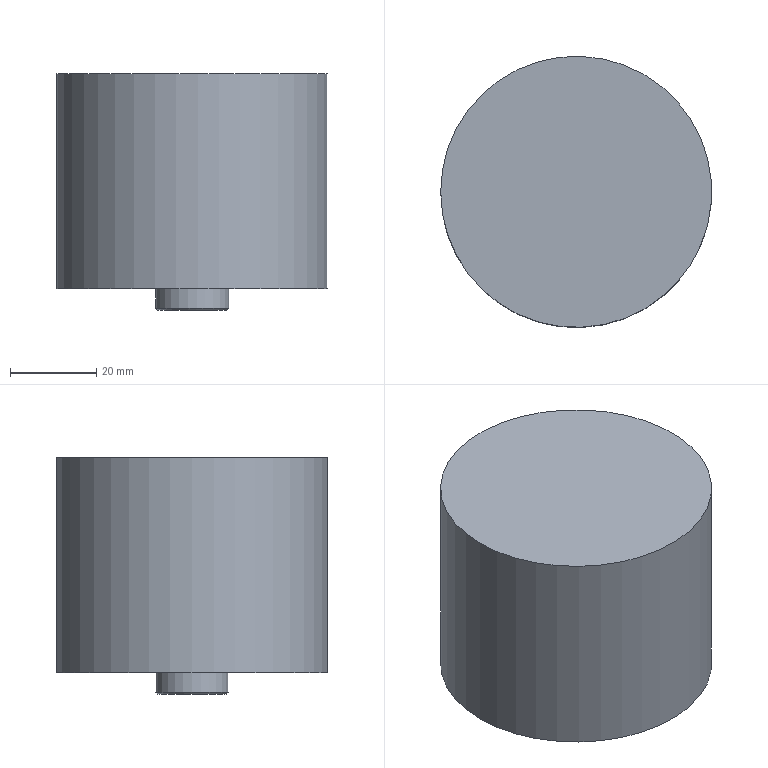Part | NX | features solid 2 | 1 solid | 6 faces | box 63 x 63 x 55 mm | volume 156991 mm3 | plane 3 | cylinder 2 | cone 1 | commonest cylinder face diameters 17 x1 63 x1
STEP:
#1=CARTESIAN_POINT('',(1143.5,-800.,-55.));
#2=VERTEX_POINT('',#1);
#3=CARTESIAN_POINT('',(1175.,-800.,-55.));
#4=DIRECTION('',(0.,0.,-1.));
#5=DIRECTION('',(-1.,0.,0.));
#6=AXIS2_PLACEMENT_3D('',#3,#4,#5);
#7=CIRCLE('',#6,31.5);
#8=EDGE_CURVE('',#2,#2,#7,.T.);
#9=ORIENTED_EDGE('',*,*,#8,.T.);
#10=EDGE_LOOP('',(#9));
#11=FACE_BOUND('',#10,.T.);
#12=CARTESIAN_POINT('',(1143.5,-800.,-105.));
#13=VERTEX_POINT('',#12);
#14=CARTESIAN_POINT('',(1175.,-800.,-105.));
#15=DIRECTION('',(0.,0.,-1.));
#16=DIRECTION('',(-1.,0.,0.));
#17=AXIS2_PLACEMENT_3D('',#14,#15,#16);
#18=CIRCLE('',#17,31.5);
#19=EDGE_CURVE('',#13,#13,#18,.T.);
#20=ORIENTED_EDGE('',*,*,#19,.F.);
#21=EDGE_LOOP('',(#20));
#22=FACE_BOUND('',#21,.T.);
#23=CARTESIAN_POINT('',(1175.,-800.,75.));
#24=DIRECTION('',(0.,0.,-1.));
#25=DIRECTION('',(1.,0.,0.));
#26=AXIS2_PLACEMENT_3D('',#23,#24,#25);
#27=CYLINDRICAL_SURFACE('',#26,31.5);
#28=ADVANCED_FACE('',(#11,#22),#27,.T.);
#29=ORIENTED_EDGE('',*,*,#8,.F.);
#30=EDGE_LOOP('',(#29));
#31=FACE_BOUND('',#30,.T.);
#32=CARTESIAN_POINT('',(1175.,-800.,-55.));
#33=DIRECTION('',(0.,0.,1.));
#34=DIRECTION('',(-1.,0.,0.));
#35=AXIS2_PLACEMENT_3D('',#32,#33,#34);
#36=PLANE('',#35);
#37=ADVANCED_FACE('',(#31),#36,.T.);
#38=CARTESIAN_POINT('',(1183.5,-800.,-105.));
#39=VERTEX_POINT('',#38);
#40=CARTESIAN_POINT('',(1175.,-800.,-105.));
#41=DIRECTION('',(0.,0.,1.));
#42=DIRECTION('',(1.,0.,0.));
#43=AXIS2_PLACEMENT_3D('',#40,#41,#42);
#44=CIRCLE('',#43,8.5);
#45=EDGE_CURVE('',#39,#39,#44,.T.);
#46=ORIENTED_EDGE('',*,*,#45,.T.);
#47=EDGE_LOOP('',(#46));
#48=FACE_BOUND('',#47,.T.);
#49=ORIENTED_EDGE('',*,*,#19,.T.);
#50=EDGE_LOOP('',(#49));
#51=FACE_BOUND('',#50,.T.);
#52=CARTESIAN_POINT('',(1175.,-800.,-105.));
#53=DIRECTION('',(0.,0.,1.));
#54=DIRECTION('',(-1.,0.,0.));
#55=AXIS2_PLACEMENT_3D('',#52,#53,#54);
#56=PLANE('',#55);
#57=ADVANCED_FACE('',(#48,#51),#56,.F.);
#58=CARTESIAN_POINT('',(1183.,-800.,-110.));
#59=VERTEX_POINT('',#58);
#60=CARTESIAN_POINT('',(1175.,-800.,-110.));
#61=DIRECTION('',(0.,0.,1.));
#62=DIRECTION('',(1.,0.,0.));
#63=AXIS2_PLACEMENT_3D('',#60,#61,#62);
#64=CIRCLE('',#63,8.);
#65=EDGE_CURVE('',#59,#59,#64,.T.);
#66=ORIENTED_EDGE('',*,*,#65,.F.);
#67=EDGE_LOOP('',(#66));
#68=FACE_BOUND('',#67,.T.);
#69=CARTESIAN_POINT('',(1175.,-800.,-110.));
#70=DIRECTION('',(0.,0.,-1.));
#71=DIRECTION('',(1.,0.,0.));
#72=AXIS2_PLACEMENT_3D('',#69,#70,#71);
#73=PLANE('',#72);
#74=ADVANCED_FACE('',(#68),#73,.T.);
#75=CARTESIAN_POINT('',(1183.5,-800.,-109.5));
#76=VERTEX_POINT('',#75);
#77=CARTESIAN_POINT('',(1175.,-800.,-109.5));
#78=DIRECTION('',(0.,0.,1.));
#79=DIRECTION('',(1.,0.,0.));
#80=AXIS2_PLACEMENT_3D('',#77,#78,#79);
#81=CIRCLE('',#80,8.5);
#82=EDGE_CURVE('',#76,#76,#81,.F.);
#83=ORIENTED_EDGE('',*,*,#82,.F.);
#84=EDGE_LOOP('',(#83));
#85=FACE_BOUND('',#84,.T.);
#86=ORIENTED_EDGE('',*,*,#45,.F.);
#87=EDGE_LOOP('',(#86));
#88=FACE_BOUND('',#87,.T.);
#89=CARTESIAN_POINT('',(1175.,-800.,-105.));
#90=DIRECTION('',(0.,0.,-1.));
#91=DIRECTION('',(1.,0.,0.));
#92=AXIS2_PLACEMENT_3D('',#89,#90,#91);
#93=CYLINDRICAL_SURFACE('',#92,8.5);
#94=ADVANCED_FACE('',(#85,#88),#93,.T.);
#95=ORIENTED_EDGE('',*,*,#82,.T.);
#96=EDGE_LOOP('',(#95));
#97=FACE_BOUND('',#96,.T.);
#98=ORIENTED_EDGE('',*,*,#65,.T.);
#99=EDGE_LOOP('',(#98));
#100=FACE_BOUND('',#99,.T.);
#101=CARTESIAN_POINT('',(1175.,-800.,-110.));
#102=DIRECTION('',(0.,0.,1.));
#103=DIRECTION('',(-1.,0.,0.));
#104=AXIS2_PLACEMENT_3D('',#101,#102,#103);
#105=CONICAL_SURFACE('',#104,8.,0.7854);
#106=ADVANCED_FACE('',(#97,#100),#105,.T.);
#107=CLOSED_SHELL('',(#28,#37,#57,#74,#94,#106));
#108=MANIFOLD_SOLID_BREP('',#107);
#109=(LENGTH_UNIT()NAMED_UNIT(*)SI_UNIT(.MILLI.,.METRE.));
#110=UNCERTAINTY_MEASURE_WITH_UNIT(LENGTH_MEASURE(0.00001),#109,'','');
#111=(NAMED_UNIT(*)PLANE_ANGLE_UNIT()SI_UNIT($,.RADIAN.));
#112=(NAMED_UNIT(*)SI_UNIT($,.STERADIAN.)SOLID_ANGLE_UNIT());
#113=(GEOMETRIC_REPRESENTATION_CONTEXT(3)GLOBAL_UNCERTAINTY_ASSIGNED_CONTEXT((#110))GLOBAL_UNIT_ASSIGNED_CONTEXT((#109,#111,#112))REPRESENTATION_CONTEXT('',''));
#114=ADVANCED_BREP_SHAPE_REPRESENTATION('',(#108),#113);